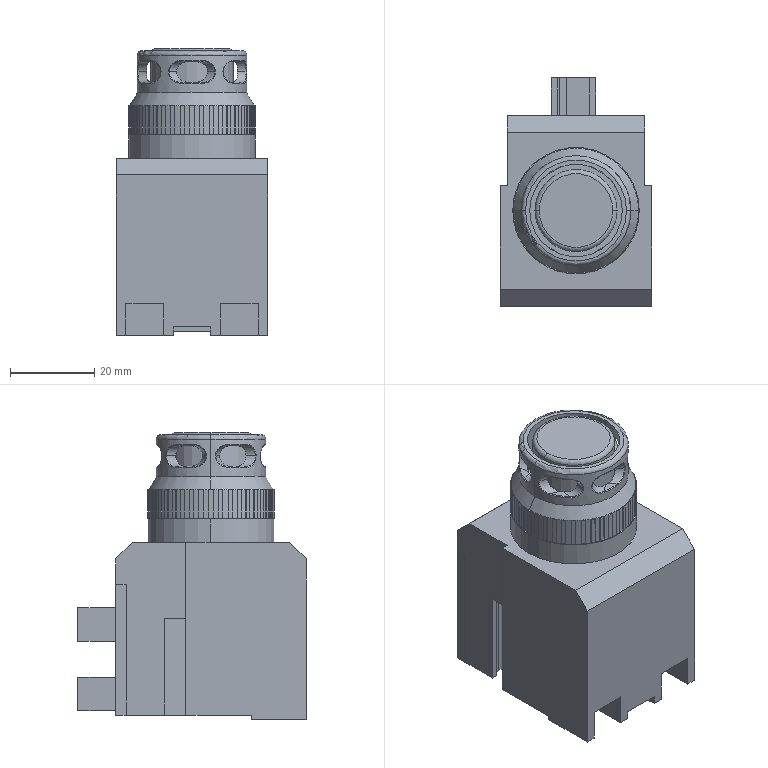Part | STEP file | push_lamp1 | 6 solids | 360 faces | box 36 x 54.3 x 68.1 mm | volume 76407 mm3 | plane 280 | cylinder 38 | spline 24 | torus 16 | cone 2 | commonest cylinder face diameters 5 x24 3.979 x4 19.5 x2 22 x2 26 x2 29.6 x2